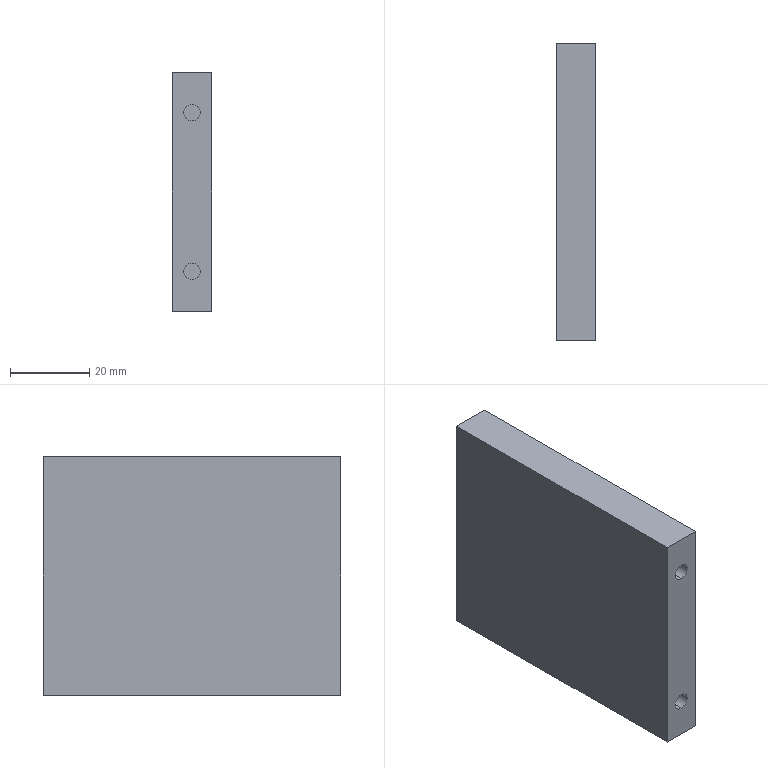Part | STEP file | 0246_203_Plate | 1 solid | 12 faces | box 10 x 75 x 60 mm | volume 44656 mm3 | plane 8 | cylinder 4 | commonest cylinder face diameters 4.2 x4
STEP:
#1=CARTESIAN_POINT('',(0.,0.,0.));
#2=DIRECTION('',(0.,0.,1.));
#3=DIRECTION('',(1.,0.,0.));
#4=AXIS2_PLACEMENT_3D('',#1,#2,#3);
#5=CARTESIAN_POINT('',(5.,12.4,17.9));
#6=VERTEX_POINT('',#5);
#7=CARTESIAN_POINT('',(5.,0.,17.9));
#8=VERTEX_POINT('',#7);
#9=CARTESIAN_POINT('',(5.,0.,17.9));
#10=DIRECTION('',(0.,-1.,0.));
#11=VECTOR('',#10,1.);
#12=LINE('',#9,#11);
#13=CARTESIAN_POINT('',(5.,0.,20.));
#14=DIRECTION('',(0.,-1.,0.));
#15=DIRECTION('',(0.,0.,-1.));
#16=AXIS2_PLACEMENT_3D('',#13,#14,#15);
#17=CYLINDRICAL_SURFACE('',#16,2.1);
#18=CARTESIAN_POINT('',(6.283,0.));
#19=DIRECTION('',(0.,1.));
#20=VECTOR('',#19,1.);
#21=LINE('',#18,#20);
#22=(GEOMETRIC_REPRESENTATION_CONTEXT(2)PARAMETRIC_REPRESENTATION_CONTEXT()REPRESENTATION_CONTEXT('',''));
#23=DEFINITIONAL_REPRESENTATION('',(#21),#22);
#24=PCURVE('',#17,#23);
#25=CARTESIAN_POINT('',(5.,0.,20.));
#26=DIRECTION('',(0.,-1.,0.));
#27=DIRECTION('',(0.,0.,-1.));
#28=AXIS2_PLACEMENT_3D('',#25,#26,#27);
#29=CYLINDRICAL_SURFACE('',#28,2.1);
#30=CARTESIAN_POINT('',(0.,0.));
#31=DIRECTION('',(0.,1.));
#32=VECTOR('',#31,1.);
#33=LINE('',#30,#32);
#34=(GEOMETRIC_REPRESENTATION_CONTEXT(2)PARAMETRIC_REPRESENTATION_CONTEXT()REPRESENTATION_CONTEXT('',''));
#35=DEFINITIONAL_REPRESENTATION('',(#33),#34);
#36=PCURVE('',#29,#35);
#37=SURFACE_CURVE('',#12,(#24,#36),.PCURVE_S1.);
#38=EDGE_CURVE('',#6,#8,#37,.T.);
#39=ORIENTED_EDGE('',*,*,#38,.T.);
#40=CARTESIAN_POINT('',(5.,0.,22.1));
#41=VERTEX_POINT('',#40);
#42=CARTESIAN_POINT('',(5.,0.,20.));
#43=DIRECTION('',(0.,-1.,0.));
#44=DIRECTION('',(0.,0.,-1.));
#45=AXIS2_PLACEMENT_3D('',#42,#43,#44);
#46=CIRCLE('',#45,2.1);
#47=CARTESIAN_POINT('',(0.,0.));
#48=DIRECTION('',(1.,0.));
#49=VECTOR('',#48,1.);
#50=LINE('',#47,#49);
#51=(GEOMETRIC_REPRESENTATION_CONTEXT(2)PARAMETRIC_REPRESENTATION_CONTEXT()REPRESENTATION_CONTEXT('',''));
#52=DEFINITIONAL_REPRESENTATION('',(#50),#51);
#53=PCURVE('',#17,#52);
#54=CARTESIAN_POINT('',(10.,0.,30.));
#55=DIRECTION('',(0.,1.,0.));
#56=DIRECTION('',(0.,0.,1.));
#57=AXIS2_PLACEMENT_3D('',#54,#55,#56);
#58=PLANE('',#57);
#59=CARTESIAN_POINT('',(-12.1,-5.));
#60=CARTESIAN_POINT('',(-12.1,-1.363));
#61=CARTESIAN_POINT('',(-8.95,-3.181));
#62=CARTESIAN_POINT('',(-5.8,-5.));
#63=CARTESIAN_POINT('',(-8.95,-6.819));
#64=CARTESIAN_POINT('',(-12.1,-8.637));
#65=CARTESIAN_POINT('',(-12.1,-5.));
#66=(BOUNDED_CURVE()B_SPLINE_CURVE(2,(#59,#60,#61,#62,#63,#64,#65),.UNSPECIFIED.,.T.,.F.)B_SPLINE_CURVE_WITH_KNOTS((1,2,2,2,2,1),(-2.094,0.,2.094,4.189,6.283,8.378),.UNSPECIFIED.)CURVE()GEOMETRIC_REPRESENTATION_ITEM()RATIONAL_B_SPLINE_CURVE((1.,0.5,1.,0.5,1.,0.5,1.))REPRESENTATION_ITEM(''));
#67=(GEOMETRIC_REPRESENTATION_CONTEXT(2)PARAMETRIC_REPRESENTATION_CONTEXT()REPRESENTATION_CONTEXT('',''));
#68=DEFINITIONAL_REPRESENTATION('',(#66),#67);
#69=PCURVE('',#58,#68);
#70=SURFACE_CURVE('',#46,(#53,#69),.PCURVE_S1.);
#71=EDGE_CURVE('',#41,#8,#70,.T.);
#72=ORIENTED_EDGE('',*,*,#71,.F.);
#73=CARTESIAN_POINT('',(5.,12.4,22.1));
#74=VERTEX_POINT('',#73);
#75=CARTESIAN_POINT('',(5.,0.,22.1));
#76=DIRECTION('',(0.,-1.,0.));
#77=VECTOR('',#76,1.);
#78=LINE('',#75,#77);
#79=CARTESIAN_POINT('',(3.142,0.));
#80=DIRECTION('',(0.,1.));
#81=VECTOR('',#80,1.);
#82=LINE('',#79,#81);
#83=(GEOMETRIC_REPRESENTATION_CONTEXT(2)PARAMETRIC_REPRESENTATION_CONTEXT()REPRESENTATION_CONTEXT('',''));
#84=DEFINITIONAL_REPRESENTATION('',(#82),#83);
#85=PCURVE('',#17,#84);
#86=CARTESIAN_POINT('',(3.142,0.));
#87=DIRECTION('',(0.,1.));
#88=VECTOR('',#87,1.);
#89=LINE('',#86,#88);
#90=(GEOMETRIC_REPRESENTATION_CONTEXT(2)PARAMETRIC_REPRESENTATION_CONTEXT()REPRESENTATION_CONTEXT('',''));
#91=DEFINITIONAL_REPRESENTATION('',(#89),#90);
#92=PCURVE('',#29,#91);
#93=SURFACE_CURVE('',#78,(#85,#92),.PCURVE_S1.);
#94=EDGE_CURVE('',#74,#41,#93,.T.);
#95=ORIENTED_EDGE('',*,*,#94,.F.);
#96=CARTESIAN_POINT('',(5.,12.4,20.));
#97=DIRECTION('',(0.,-1.,0.));
#98=DIRECTION('',(0.,0.,-1.));
#99=AXIS2_PLACEMENT_3D('',#96,#97,#98);
#100=CIRCLE('',#99,2.1);
#101=CARTESIAN_POINT('',(0.,-12.4));
#102=DIRECTION('',(1.,0.));
#103=VECTOR('',#102,1.);
#104=LINE('',#101,#103);
#105=(GEOMETRIC_REPRESENTATION_CONTEXT(2)PARAMETRIC_REPRESENTATION_CONTEXT()REPRESENTATION_CONTEXT('',''));
#106=DEFINITIONAL_REPRESENTATION('',(#104),#105);
#107=PCURVE('',#17,#106);
#108=CARTESIAN_POINT('',(5.,12.4,20.));
#109=DIRECTION('',(0.,1.,0.));
#110=DIRECTION('',(0.,0.,1.));
#111=AXIS2_PLACEMENT_3D('',#108,#109,#110);
#112=PLANE('',#111);
#113=CARTESIAN_POINT('',(-2.1,0.));
#114=CARTESIAN_POINT('',(-2.1,3.637));
#115=CARTESIAN_POINT('',(1.05,1.819));
#116=CARTESIAN_POINT('',(4.2,0.));
#117=CARTESIAN_POINT('',(1.05,-1.819));
#118=CARTESIAN_POINT('',(-2.1,-3.637));
#119=CARTESIAN_POINT('',(-2.1,0.));
#120=(BOUNDED_CURVE()B_SPLINE_CURVE(2,(#113,#114,#115,#116,#117,#118,#119),.UNSPECIFIED.,.T.,.F.)B_SPLINE_CURVE_WITH_KNOTS((1,2,2,2,2,1),(-2.094,0.,2.094,4.189,6.283,8.378),.UNSPECIFIED.)CURVE()GEOMETRIC_REPRESENTATION_ITEM()RATIONAL_B_SPLINE_CURVE((1.,0.5,1.,0.5,1.,0.5,1.))REPRESENTATION_ITEM(''));
#121=(GEOMETRIC_REPRESENTATION_CONTEXT(2)PARAMETRIC_REPRESENTATION_CONTEXT()REPRESENTATION_CONTEXT('',''));
#122=DEFINITIONAL_REPRESENTATION('',(#120),#121);
#123=PCURVE('',#112,#122);
#124=SURFACE_CURVE('',#100,(#107,#123),.PCURVE_S1.);
#125=EDGE_CURVE('',#74,#6,#124,.T.);
#126=ORIENTED_EDGE('',*,*,#125,.T.);
#127=EDGE_LOOP('',(#39,#72,#95,#126));
#128=FACE_BOUND('',#127,.F.);
#129=ADVANCED_FACE('',(#128),#17,.F.);
#130=CARTESIAN_POINT('',(5.,12.4,-22.1));
#131=VERTEX_POINT('',#130);
#132=CARTESIAN_POINT('',(5.,0.,-22.1));
#133=VERTEX_POINT('',#132);
#134=CARTESIAN_POINT('',(5.,0.,-22.1));
#135=DIRECTION('',(0.,-1.,0.));
#136=VECTOR('',#135,1.);
#137=LINE('',#134,#136);
#138=CARTESIAN_POINT('',(5.,0.,-20.));
#139=DIRECTION('',(0.,-1.,0.));
#140=DIRECTION('',(0.,0.,-1.));
#141=AXIS2_PLACEMENT_3D('',#138,#139,#140);
#142=CYLINDRICAL_SURFACE('',#141,2.1);
#143=CARTESIAN_POINT('',(6.283,0.));
#144=DIRECTION('',(0.,1.));
#145=VECTOR('',#144,1.);
#146=LINE('',#143,#145);
#147=(GEOMETRIC_REPRESENTATION_CONTEXT(2)PARAMETRIC_REPRESENTATION_CONTEXT()REPRESENTATION_CONTEXT('',''));
#148=DEFINITIONAL_REPRESENTATION('',(#146),#147);
#149=PCURVE('',#142,#148);
#150=CARTESIAN_POINT('',(5.,0.,-20.));
#151=DIRECTION('',(0.,-1.,0.));
#152=DIRECTION('',(0.,0.,-1.));
#153=AXIS2_PLACEMENT_3D('',#150,#151,#152);
#154=CYLINDRICAL_SURFACE('',#153,2.1);
#155=CARTESIAN_POINT('',(0.,0.));
#156=DIRECTION('',(0.,1.));
#157=VECTOR('',#156,1.);
#158=LINE('',#155,#157);
#159=(GEOMETRIC_REPRESENTATION_CONTEXT(2)PARAMETRIC_REPRESENTATION_CONTEXT()REPRESENTATION_CONTEXT('',''));
#160=DEFINITIONAL_REPRESENTATION('',(#158),#159);
#161=PCURVE('',#154,#160);
#162=SURFACE_CURVE('',#137,(#149,#161),.PCURVE_S1.);
#163=EDGE_CURVE('',#131,#133,#162,.T.);
#164=ORIENTED_EDGE('',*,*,#163,.T.);
#165=CARTESIAN_POINT('',(5.,0.,-17.9));
#166=VERTEX_POINT('',#165);
#167=CARTESIAN_POINT('',(5.,0.,-20.));
#168=DIRECTION('',(0.,-1.,0.));
#169=DIRECTION('',(0.,0.,-1.));
#170=AXIS2_PLACEMENT_3D('',#167,#168,#169);
#171=CIRCLE('',#170,2.1);
#172=CARTESIAN_POINT('',(0.,0.));
#173=DIRECTION('',(1.,0.));
#174=VECTOR('',#173,1.);
#175=LINE('',#172,#174);
#176=(GEOMETRIC_REPRESENTATION_CONTEXT(2)PARAMETRIC_REPRESENTATION_CONTEXT()REPRESENTATION_CONTEXT('',''));
#177=DEFINITIONAL_REPRESENTATION('',(#175),#176);
#178=PCURVE('',#142,#177);
#179=CARTESIAN_POINT('',(-52.1,-5.));
#180=CARTESIAN_POINT('',(-52.1,-1.363));
#181=CARTESIAN_POINT('',(-48.95,-3.181));
#182=CARTESIAN_POINT('',(-45.8,-5.));
#183=CARTESIAN_POINT('',(-48.95,-6.819));
#184=CARTESIAN_POINT('',(-52.1,-8.637));
#185=CARTESIAN_POINT('',(-52.1,-5.));
#186=(BOUNDED_CURVE()B_SPLINE_CURVE(2,(#179,#180,#181,#182,#183,#184,#185),.UNSPECIFIED.,.T.,.F.)B_SPLINE_CURVE_WITH_KNOTS((1,2,2,2,2,1),(-2.094,0.,2.094,4.189,6.283,8.378),.UNSPECIFIED.)CURVE()GEOMETRIC_REPRESENTATION_ITEM()RATIONAL_B_SPLINE_CURVE((1.,0.5,1.,0.5,1.,0.5,1.))REPRESENTATION_ITEM(''));
#187=(GEOMETRIC_REPRESENTATION_CONTEXT(2)PARAMETRIC_REPRESENTATION_CONTEXT()REPRESENTATION_CONTEXT('',''));
#188=DEFINITIONAL_REPRESENTATION('',(#186),#187);
#189=PCURVE('',#58,#188);
#190=SURFACE_CURVE('',#171,(#178,#189),.PCURVE_S1.);
#191=EDGE_CURVE('',#166,#133,#190,.T.);
#192=ORIENTED_EDGE('',*,*,#191,.F.);
#193=CARTESIAN_POINT('',(5.,12.4,-17.9));
#194=VERTEX_POINT('',#193);
#195=CARTESIAN_POINT('',(5.,0.,-17.9));
#196=DIRECTION('',(0.,-1.,0.));
#197=VECTOR('',#196,1.);
#198=LINE('',#195,#197);
#199=CARTESIAN_POINT('',(3.142,0.));
#200=DIRECTION('',(0.,1.));
#201=VECTOR('',#200,1.);
#202=LINE('',#199,#201);
#203=(GEOMETRIC_REPRESENTATION_CONTEXT(2)PARAMETRIC_REPRESENTATION_CONTEXT()REPRESENTATION_CONTEXT('',''));
#204=DEFINITIONAL_REPRESENTATION('',(#202),#203);
#205=PCURVE('',#142,#204);
#206=CARTESIAN_POINT('',(3.142,0.));
#207=DIRECTION('',(0.,1.));
#208=VECTOR('',#207,1.);
#209=LINE('',#206,#208);
#210=(GEOMETRIC_REPRESENTATION_CONTEXT(2)PARAMETRIC_REPRESENTATION_CONTEXT()REPRESENTATION_CONTEXT('',''));
#211=DEFINITIONAL_REPRESENTATION('',(#209),#210);
#212=PCURVE('',#154,#211);
#213=SURFACE_CURVE('',#198,(#205,#212),.PCURVE_S1.);
#214=EDGE_CURVE('',#194,#166,#213,.T.);
#215=ORIENTED_EDGE('',*,*,#214,.F.);
#216=CARTESIAN_POINT('',(5.,12.4,-20.));
#217=DIRECTION('',(0.,-1.,0.));
#218=DIRECTION('',(0.,0.,-1.));
#219=AXIS2_PLACEMENT_3D('',#216,#217,#218);
#220=CIRCLE('',#219,2.1);
#221=CARTESIAN_POINT('',(0.,-12.4));
#222=DIRECTION('',(1.,0.));
#223=VECTOR('',#222,1.);
#224=LINE('',#221,#223);
#225=(GEOMETRIC_REPRESENTATION_CONTEXT(2)PARAMETRIC_REPRESENTATION_CONTEXT()REPRESENTATION_CONTEXT('',''));
#226=DEFINITIONAL_REPRESENTATION('',(#224),#225);
#227=PCURVE('',#142,#226);
#228=CARTESIAN_POINT('',(5.,12.4,-20.));
#229=DIRECTION('',(0.,1.,0.));
#230=DIRECTION('',(0.,0.,1.));
#231=AXIS2_PLACEMENT_3D('',#228,#229,#230);
#232=PLANE('',#231);
#233=CARTESIAN_POINT('',(-2.1,0.));
#234=CARTESIAN_POINT('',(-2.1,3.637));
#235=CARTESIAN_POINT('',(1.05,1.819));
#236=CARTESIAN_POINT('',(4.2,0.));
#237=CARTESIAN_POINT('',(1.05,-1.819));
#238=CARTESIAN_POINT('',(-2.1,-3.637));
#239=CARTESIAN_POINT('',(-2.1,0.));
#240=(BOUNDED_CURVE()B_SPLINE_CURVE(2,(#233,#234,#235,#236,#237,#238,#239),.UNSPECIFIED.,.T.,.F.)B_SPLINE_CURVE_WITH_KNOTS((1,2,2,2,2,1),(-2.094,0.,2.094,4.189,6.283,8.378),.UNSPECIFIED.)CURVE()GEOMETRIC_REPRESENTATION_ITEM()RATIONAL_B_SPLINE_CURVE((1.,0.5,1.,0.5,1.,0.5,1.))REPRESENTATION_ITEM(''));
#241=(GEOMETRIC_REPRESENTATION_CONTEXT(2)PARAMETRIC_REPRESENTATION_CONTEXT()REPRESENTATION_CONTEXT('',''));
#242=DEFINITIONAL_REPRESENTATION('',(#240),#241);
#243=PCURVE('',#232,#242);
#244=SURFACE_CURVE('',#220,(#227,#243),.PCURVE_S1.);
#245=EDGE_CURVE('',#194,#131,#244,.T.);
#246=ORIENTED_EDGE('',*,*,#245,.T.);
#247=EDGE_LOOP('',(#164,#192,#215,#246));
#248=FACE_BOUND('',#247,.F.);
#249=ADVANCED_FACE('',(#248),#142,.F.);
#250=CARTESIAN_POINT('',(0.,75.,30.));
#251=VERTEX_POINT('',#250);
#252=CARTESIAN_POINT('',(0.,0.,30.));
#253=VERTEX_POINT('',#252);
#254=CARTESIAN_POINT('',(0.,75.,30.));
#255=DIRECTION('',(0.,-1.,0.));
#256=VECTOR('',#255,1.);
#257=LINE('',#254,#256);
#258=CARTESIAN_POINT('',(10.,75.,30.));
#259=DIRECTION('',(0.,0.,-1.));
#260=DIRECTION('',(0.,1.,0.));
#261=AXIS2_PLACEMENT_3D('',#258,#259,#260);
#262=PLANE('',#261);
#263=CARTESIAN_POINT('',(0.,-10.));
#264=DIRECTION('',(-1.,0.));
#265=VECTOR('',#264,1.);
#266=LINE('',#263,#265);
#267=(GEOMETRIC_REPRESENTATION_CONTEXT(2)PARAMETRIC_REPRESENTATION_CONTEXT()REPRESENTATION_CONTEXT('',''));
#268=DEFINITIONAL_REPRESENTATION('',(#266),#267);
#269=PCURVE('',#262,#268);
#270=CARTESIAN_POINT('',(0.,0.,30.));
#271=DIRECTION('',(1.,0.,0.));
#272=DIRECTION('',(0.,0.,-1.));
#273=AXIS2_PLACEMENT_3D('',#270,#271,#272);
#274=PLANE('',#273);
#275=CARTESIAN_POINT('',(0.,75.));
#276=DIRECTION('',(0.,-1.));
#277=VECTOR('',#276,1.);
#278=LINE('',#275,#277);
#279=(GEOMETRIC_REPRESENTATION_CONTEXT(2)PARAMETRIC_REPRESENTATION_CONTEXT()REPRESENTATION_CONTEXT('',''));
#280=DEFINITIONAL_REPRESENTATION('',(#278),#279);
#281=PCURVE('',#274,#280);
#282=SURFACE_CURVE('',#257,(#269,#281),.PCURVE_S1.);
#283=EDGE_CURVE('',#251,#253,#282,.T.);
#284=ORIENTED_EDGE('',*,*,#283,.T.);
#285=CARTESIAN_POINT('',(10.,0.,30.));
#286=VERTEX_POINT('',#285);
#287=CARTESIAN_POINT('',(10.,0.,30.));
#288=DIRECTION('',(-1.,0.,0.));
#289=VECTOR('',#288,1.);
#290=LINE('',#287,#289);
#291=CARTESIAN_POINT('',(-75.,0.));
#292=DIRECTION('',(0.,-1.));
#293=VECTOR('',#292,1.);
#294=LINE('',#291,#293);
#295=(GEOMETRIC_REPRESENTATION_CONTEXT(2)PARAMETRIC_REPRESENTATION_CONTEXT()REPRESENTATION_CONTEXT('',''));
#296=DEFINITIONAL_REPRESENTATION('',(#294),#295);
#297=PCURVE('',#262,#296);
#298=CARTESIAN_POINT('',(0.,0.));
#299=DIRECTION('',(0.,-1.));
#300=VECTOR('',#299,1.);
#301=LINE('',#298,#300);
#302=(GEOMETRIC_REPRESENTATION_CONTEXT(2)PARAMETRIC_REPRESENTATION_CONTEXT()REPRESENTATION_CONTEXT('',''));
#303=DEFINITIONAL_REPRESENTATION('',(#301),#302);
#304=PCURVE('',#58,#303);
#305=SURFACE_CURVE('',#290,(#297,#304),.PCURVE_S1.);
#306=EDGE_CURVE('',#286,#253,#305,.T.);
#307=ORIENTED_EDGE('',*,*,#306,.F.);
#308=CARTESIAN_POINT('',(10.,75.,30.));
#309=VERTEX_POINT('',#308);
#310=CARTESIAN_POINT('',(10.,75.,30.));
#311=DIRECTION('',(0.,-1.,0.));
#312=VECTOR('',#311,1.);
#313=LINE('',#310,#312);
#314=CARTESIAN_POINT('',(0.,0.));
#315=DIRECTION('',(-1.,0.));
#316=VECTOR('',#315,1.);
#317=LINE('',#314,#316);
#318=(GEOMETRIC_REPRESENTATION_CONTEXT(2)PARAMETRIC_REPRESENTATION_CONTEXT()REPRESENTATION_CONTEXT('',''));
#319=DEFINITIONAL_REPRESENTATION('',(#317),#318);
#320=PCURVE('',#262,#319);
#321=CARTESIAN_POINT('',(10.,0.,30.));
#322=DIRECTION('',(1.,0.,0.));
#323=DIRECTION('',(0.,0.,-1.));
#324=AXIS2_PLACEMENT_3D('',#321,#322,#323);
#325=PLANE('',#324);
#326=CARTESIAN_POINT('',(0.,75.));
#327=DIRECTION('',(0.,-1.));
#328=VECTOR('',#327,1.);
#329=LINE('',#326,#328);
#330=(GEOMETRIC_REPRESENTATION_CONTEXT(2)PARAMETRIC_REPRESENTATION_CONTEXT()REPRESENTATION_CONTEXT('',''));
#331=DEFINITIONAL_REPRESENTATION('',(#329),#330);
#332=PCURVE('',#325,#331);
#333=SURFACE_CURVE('',#313,(#320,#332),.PCURVE_S1.);
#334=EDGE_CURVE('',#309,#286,#333,.T.);
#335=ORIENTED_EDGE('',*,*,#334,.F.);
#336=CARTESIAN_POINT('',(10.,75.,30.));
#337=DIRECTION('',(-1.,0.,0.));
#338=VECTOR('',#337,1.);
#339=LINE('',#336,#338);
#340=CARTESIAN_POINT('',(0.,0.));
#341=DIRECTION('',(0.,-1.));
#342=VECTOR('',#341,1.);
#343=LINE('',#340,#342);
#344=(GEOMETRIC_REPRESENTATION_CONTEXT(2)PARAMETRIC_REPRESENTATION_CONTEXT()REPRESENTATION_CONTEXT('',''));
#345=DEFINITIONAL_REPRESENTATION('',(#343),#344);
#346=PCURVE('',#262,#345);
#347=CARTESIAN_POINT('',(10.,75.,30.));
#348=DIRECTION('',(0.,-1.,0.));
#349=DIRECTION('',(0.,0.,-1.));
#350=AXIS2_PLACEMENT_3D('',#347,#348,#349);
#351=PLANE('',#350);
#352=CARTESIAN_POINT('',(0.,0.));
#353=DIRECTION('',(0.,-1.));
#354=VECTOR('',#353,1.);
#355=LINE('',#352,#354);
#356=(GEOMETRIC_REPRESENTATION_CONTEXT(2)PARAMETRIC_REPRESENTATION_CONTEXT()REPRESENTATION_CONTEXT('',''));
#357=DEFINITIONAL_REPRESENTATION('',(#355),#356);
#358=PCURVE('',#351,#357);
#359=SURFACE_CURVE('',#339,(#346,#358),.PCURVE_S1.);
#360=EDGE_CURVE('',#309,#251,#359,.T.);
#361=ORIENTED_EDGE('',*,*,#360,.T.);
#362=EDGE_LOOP('',(#284,#307,#335,#361));
#363=FACE_BOUND('',#362,.T.);
#364=ADVANCED_FACE('',(#363),#262,.F.);
#365=CARTESIAN_POINT('',(5.,0.,20.));
#366=DIRECTION('',(0.,-1.,0.));
#367=DIRECTION('',(0.,0.,-1.));
#368=AXIS2_PLACEMENT_3D('',#365,#366,#367);
#369=CIRCLE('',#368,2.1);
#370=CARTESIAN_POINT('',(-12.1,-5.));
#371=CARTESIAN_POINT('',(-12.1,-1.363));
#372=CARTESIAN_POINT('',(-8.95,-3.181));
#373=CARTESIAN_POINT('',(-5.8,-5.));
#374=CARTESIAN_POINT('',(-8.95,-6.819));
#375=CARTESIAN_POINT('',(-12.1,-8.637));
#376=CARTESIAN_POINT('',(-12.1,-5.));
#377=(BOUNDED_CURVE()B_SPLINE_CURVE(2,(#370,#371,#372,#373,#374,#375,#376),.UNSPECIFIED.,.T.,.F.)B_SPLINE_CURVE_WITH_KNOTS((1,2,2,2,2,1),(-2.094,0.,2.094,4.189,6.283,8.378),.UNSPECIFIED.)CURVE()GEOMETRIC_REPRESENTATION_ITEM()RATIONAL_B_SPLINE_CURVE((1.,0.5,1.,0.5,1.,0.5,1.))REPRESENTATION_ITEM(''));
#378=(GEOMETRIC_REPRESENTATION_CONTEXT(2)PARAMETRIC_REPRESENTATION_CONTEXT()REPRESENTATION_CONTEXT('',''));
#379=DEFINITIONAL_REPRESENTATION('',(#377),#378);
#380=PCURVE('',#58,#379);
#381=CARTESIAN_POINT('',(0.,0.));
#382=DIRECTION('',(1.,0.));
#383=VECTOR('',#382,1.);
#384=LINE('',#381,#383);
#385=(GEOMETRIC_REPRESENTATION_CONTEXT(2)PARAMETRIC_REPRESENTATION_CONTEXT()REPRESENTATION_CONTEXT('',''));
#386=DEFINITIONAL_REPRESENTATION('',(#384),#385);
#387=PCURVE('',#29,#386);
#388=SURFACE_CURVE('',#369,(#380,#387),.PCURVE_S1.);
#389=EDGE_CURVE('',#8,#41,#388,.T.);
#390=ORIENTED_EDGE('',*,*,#389,.F.);
#391=ORIENTED_EDGE('',*,*,#71,.F.);
#392=EDGE_LOOP('',(#390,#391));
#393=FACE_BOUND('',#392,.T.);
#394=CARTESIAN_POINT('',(5.,0.,-20.));
#395=DIRECTION('',(0.,-1.,0.));
#396=DIRECTION('',(0.,0.,-1.));
#397=AXIS2_PLACEMENT_3D('',#394,#395,#396);
#398=CIRCLE('',#397,2.1);
#399=CARTESIAN_POINT('',(-52.1,-5.));
#400=CARTESIAN_POINT('',(-52.1,-1.363));
#401=CARTESIAN_POINT('',(-48.95,-3.181));
#402=CARTESIAN_POINT('',(-45.8,-5.));
#403=CARTESIAN_POINT('',(-48.95,-6.819));
#404=CARTESIAN_POINT('',(-52.1,-8.637));
#405=CARTESIAN_POINT('',(-52.1,-5.));
#406=(BOUNDED_CURVE()B_SPLINE_CURVE(2,(#399,#400,#401,#402,#403,#404,#405),.UNSPECIFIED.,.T.,.F.)B_SPLINE_CURVE_WITH_KNOTS((1,2,2,2,2,1),(-2.094,0.,2.094,4.189,6.283,8.378),.UNSPECIFIED.)CURVE()GEOMETRIC_REPRESENTATION_ITEM()RATIONAL_B_SPLINE_CURVE((1.,0.5,1.,0.5,1.,0.5,1.))REPRESENTATION_ITEM(''));
#407=(GEOMETRIC_REPRESENTATION_CONTEXT(2)PARAMETRIC_REPRESENTATION_CONTEXT()REPRESENTATION_CONTEXT('',''));
#408=DEFINITIONAL_REPRESENTATION('',(#406),#407);
#409=PCURVE('',#58,#408);
#410=CARTESIAN_POINT('',(0.,0.));
#411=DIRECTION('',(1.,0.));
#412=VECTOR('',#411,1.);
#413=LINE('',#410,#412);
#414=(GEOMETRIC_REPRESENTATION_CONTEXT(2)PARAMETRIC_REPRESENTATION_CONTEXT()REPRESENTATION_CONTEXT('',''));
#415=DEFINITIONAL_REPRESENTATION('',(#413),#414);
#416=PCURVE('',#154,#415);
#417=SURFACE_CURVE('',#398,(#409,#416),.PCURVE_S1.);
#418=EDGE_CURVE('',#133,#166,#417,.T.);
#419=ORIENTED_EDGE('',*,*,#418,.F.);
#420=ORIENTED_EDGE('',*,*,#191,.F.);
#421=EDGE_LOOP('',(#419,#420));
#422=FACE_BOUND('',#421,.T.);
#423=CARTESIAN_POINT('',(0.,0.,-30.));
#424=VERTEX_POINT('',#423);
#425=CARTESIAN_POINT('',(0.,0.,30.));
#426=DIRECTION('',(0.,0.,-1.));
#427=VECTOR('',#426,1.);
#428=LINE('',#425,#427);
#429=CARTESIAN_POINT('',(0.,-10.));
#430=DIRECTION('',(-1.,0.));
#431=VECTOR('',#430,1.);
#432=LINE('',#429,#431);
#433=(GEOMETRIC_REPRESENTATION_CONTEXT(2)PARAMETRIC_REPRESENTATION_CONTEXT()REPRESENTATION_CONTEXT('',''));
#434=DEFINITIONAL_REPRESENTATION('',(#432),#433);
#435=PCURVE('',#58,#434);
#436=CARTESIAN_POINT('',(0.,0.));
#437=DIRECTION('',(1.,0.));
#438=VECTOR('',#437,1.);
#439=LINE('',#436,#438);
#440=(GEOMETRIC_REPRESENTATION_CONTEXT(2)PARAMETRIC_REPRESENTATION_CONTEXT()REPRESENTATION_CONTEXT('',''));
#441=DEFINITIONAL_REPRESENTATION('',(#439),#440);
#442=PCURVE('',#274,#441);
#443=SURFACE_CURVE('',#428,(#435,#442),.PCURVE_S1.);
#444=EDGE_CURVE('',#253,#424,#443,.T.);
#445=ORIENTED_EDGE('',*,*,#444,.T.);
#446=CARTESIAN_POINT('',(10.,0.,-30.));
#447=VERTEX_POINT('',#446);
#448=CARTESIAN_POINT('',(10.,0.,-30.));
#449=DIRECTION('',(-1.,0.,0.));
#450=VECTOR('',#449,1.);
#451=LINE('',#448,#450);
#452=CARTESIAN_POINT('',(-60.,0.));
#453=DIRECTION('',(0.,-1.));
#454=VECTOR('',#453,1.);
#455=LINE('',#452,#454);
#456=(GEOMETRIC_REPRESENTATION_CONTEXT(2)PARAMETRIC_REPRESENTATION_CONTEXT()REPRESENTATION_CONTEXT('',''));
#457=DEFINITIONAL_REPRESENTATION('',(#455),#456);
#458=PCURVE('',#58,#457);
#459=CARTESIAN_POINT('',(10.,75.,-30.));
#460=DIRECTION('',(0.,0.,1.));
#461=DIRECTION('',(0.,-1.,0.));
#462=AXIS2_PLACEMENT_3D('',#459,#460,#461);
#463=PLANE('',#462);
#464=CARTESIAN_POINT('',(75.,0.));
#465=DIRECTION('',(0.,-1.));
#466=VECTOR('',#465,1.);
#467=LINE('',#464,#466);
#468=(GEOMETRIC_REPRESENTATION_CONTEXT(2)PARAMETRIC_REPRESENTATION_CONTEXT()REPRESENTATION_CONTEXT('',''));
#469=DEFINITIONAL_REPRESENTATION('',(#467),#468);
#470=PCURVE('',#463,#469);
#471=SURFACE_CURVE('',#451,(#458,#470),.PCURVE_S1.);
#472=EDGE_CURVE('',#447,#424,#471,.T.);
#473=ORIENTED_EDGE('',*,*,#472,.F.);
#474=CARTESIAN_POINT('',(10.,0.,30.));
#475=DIRECTION('',(0.,0.,-1.));
#476=VECTOR('',#475,1.);
#477=LINE('',#474,#476);
#478=CARTESIAN_POINT('',(0.,0.));
#479=DIRECTION('',(-1.,0.));
#480=VECTOR('',#479,1.);
#481=LINE('',#478,#480);
#482=(GEOMETRIC_REPRESENTATION_CONTEXT(2)PARAMETRIC_REPRESENTATION_CONTEXT()REPRESENTATION_CONTEXT('',''));
#483=DEFINITIONAL_REPRESENTATION('',(#481),#482);
#484=PCURVE('',#58,#483);
#485=CARTESIAN_POINT('',(0.,0.));
#486=DIRECTION('',(1.,0.));
#487=VECTOR('',#486,1.);
#488=LINE('',#485,#487);
#489=(GEOMETRIC_REPRESENTATION_CONTEXT(2)PARAMETRIC_REPRESENTATION_CONTEXT()REPRESENTATION_CONTEXT('',''));
#490=DEFINITIONAL_REPRESENTATION('',(#488),#489);
#491=PCURVE('',#325,#490);
#492=SURFACE_CURVE('',#477,(#484,#491),.PCURVE_S1.);
#493=EDGE_CURVE('',#286,#447,#492,.T.);
#494=ORIENTED_EDGE('',*,*,#493,.F.);
#495=ORIENTED_EDGE('',*,*,#306,.T.);
#496=EDGE_LOOP('',(#445,#473,#494,#495));
#497=FACE_BOUND('',#496,.T.);
#498=ADVANCED_FACE('',(#393,#422,#497),#58,.F.);
#499=CARTESIAN_POINT('',(0.,75.,-30.));
#500=VERTEX_POINT('',#499);
#501=CARTESIAN_POINT('',(0.,75.,-30.));
#502=DIRECTION('',(0.,1.,0.));
#503=VECTOR('',#502,1.);
#504=LINE('',#501,#503);
#505=CARTESIAN_POINT('',(0.,-10.));
#506=DIRECTION('',(-1.,0.));
#507=VECTOR('',#506,1.);
#508=LINE('',#505,#507);
#509=(GEOMETRIC_REPRESENTATION_CONTEXT(2)PARAMETRIC_REPRESENTATION_CONTEXT()REPRESENTATION_CONTEXT('',''));
#510=DEFINITIONAL_REPRESENTATION('',(#508),#509);
#511=PCURVE('',#463,#510);
#512=CARTESIAN_POINT('',(60.,75.));
#513=DIRECTION('',(0.,1.));
#514=VECTOR('',#513,1.);
#515=LINE('',#512,#514);
#516=(GEOMETRIC_REPRESENTATION_CONTEXT(2)PARAMETRIC_REPRESENTATION_CONTEXT()REPRESENTATION_CONTEXT('',''));
#517=DEFINITIONAL_REPRESENTATION('',(#515),#516);
#518=PCURVE('',#274,#517);
#519=SURFACE_CURVE('',#504,(#511,#518),.PCURVE_S1.);
#520=EDGE_CURVE('',#424,#500,#519,.T.);
#521=ORIENTED_EDGE('',*,*,#520,.T.);
#522=CARTESIAN_POINT('',(10.,75.,-30.));
#523=VERTEX_POINT('',#522);
#524=CARTESIAN_POINT('',(10.,75.,-30.));
#525=DIRECTION('',(-1.,0.,0.));
#526=VECTOR('',#525,1.);
#527=LINE('',#524,#526);
#528=CARTESIAN_POINT('',(0.,0.));
#529=DIRECTION('',(0.,-1.));
#530=VECTOR('',#529,1.);
#531=LINE('',#528,#530);
#532=(GEOMETRIC_REPRESENTATION_CONTEXT(2)PARAMETRIC_REPRESENTATION_CONTEXT()REPRESENTATION_CONTEXT('',''));
#533=DEFINITIONAL_REPRESENTATION('',(#531),#532);
#534=PCURVE('',#463,#533);
#535=CARTESIAN_POINT('',(60.,0.));
#536=DIRECTION('',(0.,-1.));
#537=VECTOR('',#536,1.);
#538=LINE('',#535,#537);
#539=(GEOMETRIC_REPRESENTATION_CONTEXT(2)PARAMETRIC_REPRESENTATION_CONTEXT()REPRESENTATION_CONTEXT('',''));
#540=DEFINITIONAL_REPRESENTATION('',(#538),#539);
#541=PCURVE('',#351,#540);
#542=SURFACE_CURVE('',#527,(#534,#541),.PCURVE_S1.);
#543=EDGE_CURVE('',#523,#500,#542,.T.);
#544=ORIENTED_EDGE('',*,*,#543,.F.);
#545=CARTESIAN_POINT('',(10.,75.,-30.));
#546=DIRECTION('',(0.,1.,0.));
#547=VECTOR('',#546,1.);
#548=LINE('',#545,#547);
#549=CARTESIAN_POINT('',(0.,0.));
#550=DIRECTION('',(-1.,0.));
#551=VECTOR('',#550,1.);
#552=LINE('',#549,#551);
#553=(GEOMETRIC_REPRESENTATION_CONTEXT(2)PARAMETRIC_REPRESENTATION_CONTEXT()REPRESENTATION_CONTEXT('',''));
#554=DEFINITIONAL_REPRESENTATION('',(#552),#553);
#555=PCURVE('',#463,#554);
#556=CARTESIAN_POINT('',(60.,75.));
#557=DIRECTION('',(0.,1.));
#558=VECTOR('',#557,1.);
#559=LINE('',#556,#558);
#560=(GEOMETRIC_REPRESENTATION_CONTEXT(2)PARAMETRIC_REPRESENTATION_CONTEXT()REPRESENTATION_CONTEXT('',''));
#561=DEFINITIONAL_REPRESENTATION('',(#559),#560);
#562=PCURVE('',#325,#561);
#563=SURFACE_CURVE('',#548,(#555,#562),.PCURVE_S1.);
#564=EDGE_CURVE('',#447,#523,#563,.T.);
#565=ORIENTED_EDGE('',*,*,#564,.F.);
#566=ORIENTED_EDGE('',*,*,#472,.T.);
#567=EDGE_LOOP('',(#521,#544,#565,#566));
#568=FACE_BOUND('',#567,.T.);
#569=ADVANCED_FACE('',(#568),#463,.F.);
#570=CARTESIAN_POINT('',(0.,75.,30.));
#571=DIRECTION('',(0.,0.,1.));
#572=VECTOR('',#571,1.);
#573=LINE('',#570,#572);
#574=CARTESIAN_POINT('',(0.,-10.));
#575=DIRECTION('',(-1.,0.));
#576=VECTOR('',#575,1.);
#577=LINE('',#574,#576);
#578=(GEOMETRIC_REPRESENTATION_CONTEXT(2)PARAMETRIC_REPRESENTATION_CONTEXT()REPRESENTATION_CONTEXT('',''));
#579=DEFINITIONAL_REPRESENTATION('',(#577),#578);
#580=PCURVE('',#351,#579);
#581=CARTESIAN_POINT('',(0.,75.));
#582=DIRECTION('',(-1.,0.));
#583=VECTOR('',#582,1.);
#584=LINE('',#581,#583);
#585=(GEOMETRIC_REPRESENTATION_CONTEXT(2)PARAMETRIC_REPRESENTATION_CONTEXT()REPRESENTATION_CONTEXT('',''));
#586=DEFINITIONAL_REPRESENTATION('',(#584),#585);
#587=PCURVE('',#274,#586);
#588=SURFACE_CURVE('',#573,(#580,#587),.PCURVE_S1.);
#589=EDGE_CURVE('',#500,#251,#588,.T.);
#590=ORIENTED_EDGE('',*,*,#589,.T.);
#591=ORIENTED_EDGE('',*,*,#360,.F.);
#592=CARTESIAN_POINT('',(10.,75.,30.));
#593=DIRECTION('',(0.,0.,1.));
#594=VECTOR('',#593,1.);
#595=LINE('',#592,#594);
#596=CARTESIAN_POINT('',(0.,0.));
#597=DIRECTION('',(-1.,0.));
#598=VECTOR('',#597,1.);
#599=LINE('',#596,#598);
#600=(GEOMETRIC_REPRESENTATION_CONTEXT(2)PARAMETRIC_REPRESENTATION_CONTEXT()REPRESENTATION_CONTEXT('',''));
#601=DEFINITIONAL_REPRESENTATION('',(#599),#600);
#602=PCURVE('',#351,#601);
#603=CARTESIAN_POINT('',(0.,75.));
#604=DIRECTION('',(-1.,0.));
#605=VECTOR('',#604,1.);
#606=LINE('',#603,#605);
#607=(GEOMETRIC_REPRESENTATION_CONTEXT(2)PARAMETRIC_REPRESENTATION_CONTEXT()REPRESENTATION_CONTEXT('',''));
#608=DEFINITIONAL_REPRESENTATION('',(#606),#607);
#609=PCURVE('',#325,#608);
#610=SURFACE_CURVE('',#595,(#602,#609),.PCURVE_S1.);
#611=EDGE_CURVE('',#523,#309,#610,.T.);
#612=ORIENTED_EDGE('',*,*,#611,.F.);
#613=ORIENTED_EDGE('',*,*,#543,.T.);
#614=EDGE_LOOP('',(#590,#591,#612,#613));
#615=FACE_BOUND('',#614,.T.);
#616=ADVANCED_FACE('',(#615),#351,.F.);
#617=ORIENTED_EDGE('',*,*,#334,.T.);
#618=ORIENTED_EDGE('',*,*,#493,.T.);
#619=ORIENTED_EDGE('',*,*,#564,.T.);
#620=ORIENTED_EDGE('',*,*,#611,.T.);
#621=EDGE_LOOP('',(#617,#618,#619,#620));
#622=FACE_BOUND('',#621,.T.);
#623=ADVANCED_FACE('',(#622),#325,.T.);
#624=ORIENTED_EDGE('',*,*,#283,.F.);
#625=ORIENTED_EDGE('',*,*,#589,.F.);
#626=ORIENTED_EDGE('',*,*,#520,.F.);
#627=ORIENTED_EDGE('',*,*,#444,.F.);
#628=EDGE_LOOP('',(#624,#625,#626,#627));
#629=FACE_BOUND('',#628,.T.);
#630=ADVANCED_FACE('',(#629),#274,.F.);
#631=CARTESIAN_POINT('',(5.,12.4,-20.));
#632=DIRECTION('',(0.,-1.,0.));
#633=DIRECTION('',(0.,0.,-1.));
#634=AXIS2_PLACEMENT_3D('',#631,#632,#633);
#635=CIRCLE('',#634,2.1);
#636=CARTESIAN_POINT('',(-2.1,0.));
#637=CARTESIAN_POINT('',(-2.1,3.637));
#638=CARTESIAN_POINT('',(1.05,1.819));
#639=CARTESIAN_POINT('',(4.2,0.));
#640=CARTESIAN_POINT('',(1.05,-1.819));
#641=CARTESIAN_POINT('',(-2.1,-3.637));
#642=CARTESIAN_POINT('',(-2.1,0.));
#643=(BOUNDED_CURVE()B_SPLINE_CURVE(2,(#636,#637,#638,#639,#640,#641,#642),.UNSPECIFIED.,.T.,.F.)B_SPLINE_CURVE_WITH_KNOTS((1,2,2,2,2,1),(-2.094,0.,2.094,4.189,6.283,8.378),.UNSPECIFIED.)CURVE()GEOMETRIC_REPRESENTATION_ITEM()RATIONAL_B_SPLINE_CURVE((1.,0.5,1.,0.5,1.,0.5,1.))REPRESENTATION_ITEM(''));
#644=(GEOMETRIC_REPRESENTATION_CONTEXT(2)PARAMETRIC_REPRESENTATION_CONTEXT()REPRESENTATION_CONTEXT('',''));
#645=DEFINITIONAL_REPRESENTATION('',(#643),#644);
#646=PCURVE('',#232,#645);
#647=CARTESIAN_POINT('',(0.,-12.4));
#648=DIRECTION('',(1.,0.));
#649=VECTOR('',#648,1.);
#650=LINE('',#647,#649);
#651=(GEOMETRIC_REPRESENTATION_CONTEXT(2)PARAMETRIC_REPRESENTATION_CONTEXT()REPRESENTATION_CONTEXT('',''));
#652=DEFINITIONAL_REPRESENTATION('',(#650),#651);
#653=PCURVE('',#154,#652);
#654=SURFACE_CURVE('',#635,(#646,#653),.PCURVE_S1.);
#655=EDGE_CURVE('',#131,#194,#654,.T.);
#656=ORIENTED_EDGE('',*,*,#655,.T.);
#657=ORIENTED_EDGE('',*,*,#245,.T.);
#658=EDGE_LOOP('',(#656,#657));
#659=FACE_BOUND('',#658,.T.);
#660=ADVANCED_FACE('',(#659),#232,.F.);
#661=ORIENTED_EDGE('',*,*,#418,.F.);
#662=ORIENTED_EDGE('',*,*,#163,.F.);
#663=ORIENTED_EDGE('',*,*,#655,.T.);
#664=ORIENTED_EDGE('',*,*,#214,.T.);
#665=EDGE_LOOP('',(#661,#662,#663,#664));
#666=FACE_BOUND('',#665,.F.);
#667=ADVANCED_FACE('',(#666),#154,.F.);
#668=CARTESIAN_POINT('',(5.,12.4,20.));
#669=DIRECTION('',(0.,-1.,0.));
#670=DIRECTION('',(0.,0.,-1.));
#671=AXIS2_PLACEMENT_3D('',#668,#669,#670);
#672=CIRCLE('',#671,2.1);
#673=CARTESIAN_POINT('',(-2.1,0.));
#674=CARTESIAN_POINT('',(-2.1,3.637));
#675=CARTESIAN_POINT('',(1.05,1.819));
#676=CARTESIAN_POINT('',(4.2,0.));
#677=CARTESIAN_POINT('',(1.05,-1.819));
#678=CARTESIAN_POINT('',(-2.1,-3.637));
#679=CARTESIAN_POINT('',(-2.1,0.));
#680=(BOUNDED_CURVE()B_SPLINE_CURVE(2,(#673,#674,#675,#676,#677,#678,#679),.UNSPECIFIED.,.T.,.F.)B_SPLINE_CURVE_WITH_KNOTS((1,2,2,2,2,1),(-2.094,0.,2.094,4.189,6.283,8.378),.UNSPECIFIED.)CURVE()GEOMETRIC_REPRESENTATION_ITEM()RATIONAL_B_SPLINE_CURVE((1.,0.5,1.,0.5,1.,0.5,1.))REPRESENTATION_ITEM(''));
#681=(GEOMETRIC_REPRESENTATION_CONTEXT(2)PARAMETRIC_REPRESENTATION_CONTEXT()REPRESENTATION_CONTEXT('',''));
#682=DEFINITIONAL_REPRESENTATION('',(#680),#681);
#683=PCURVE('',#112,#682);
#684=CARTESIAN_POINT('',(0.,-12.4));
#685=DIRECTION('',(1.,0.));
#686=VECTOR('',#685,1.);
#687=LINE('',#684,#686);
#688=(GEOMETRIC_REPRESENTATION_CONTEXT(2)PARAMETRIC_REPRESENTATION_CONTEXT()REPRESENTATION_CONTEXT('',''));
#689=DEFINITIONAL_REPRESENTATION('',(#687),#688);
#690=PCURVE('',#29,#689);
#691=SURFACE_CURVE('',#672,(#683,#690),.PCURVE_S1.);
#692=EDGE_CURVE('',#6,#74,#691,.T.);
#693=ORIENTED_EDGE('',*,*,#692,.T.);
#694=ORIENTED_EDGE('',*,*,#125,.T.);
#695=EDGE_LOOP('',(#693,#694));
#696=FACE_BOUND('',#695,.T.);
#697=ADVANCED_FACE('',(#696),#112,.F.);
#698=ORIENTED_EDGE('',*,*,#389,.F.);
#699=ORIENTED_EDGE('',*,*,#38,.F.);
#700=ORIENTED_EDGE('',*,*,#692,.T.);
#701=ORIENTED_EDGE('',*,*,#94,.T.);
#702=EDGE_LOOP('',(#698,#699,#700,#701));
#703=FACE_BOUND('',#702,.F.);
#704=ADVANCED_FACE('',(#703),#29,.F.);
#705=CLOSED_SHELL('',(#129,#249,#364,#498,#569,#616,#623,#630,#660,#667,#697,#704));
#706=MANIFOLD_SOLID_BREP('',#705);
#707=(LENGTH_UNIT()NAMED_UNIT(*)SI_UNIT(.MILLI.,.METRE.));
#708=UNCERTAINTY_MEASURE_WITH_UNIT(LENGTH_MEASURE(0.0000001),#707,'','');
#709=(NAMED_UNIT(*)PLANE_ANGLE_UNIT()SI_UNIT($,.RADIAN.));
#710=(NAMED_UNIT(*)SI_UNIT($,.STERADIAN.)SOLID_ANGLE_UNIT());
#711=(GEOMETRIC_REPRESENTATION_CONTEXT(3)GLOBAL_UNCERTAINTY_ASSIGNED_CONTEXT((#708))GLOBAL_UNIT_ASSIGNED_CONTEXT((#707,#709,#710))REPRESENTATION_CONTEXT('',''));
#712=ADVANCED_BREP_SHAPE_REPRESENTATION('',(#4,#706),#711);